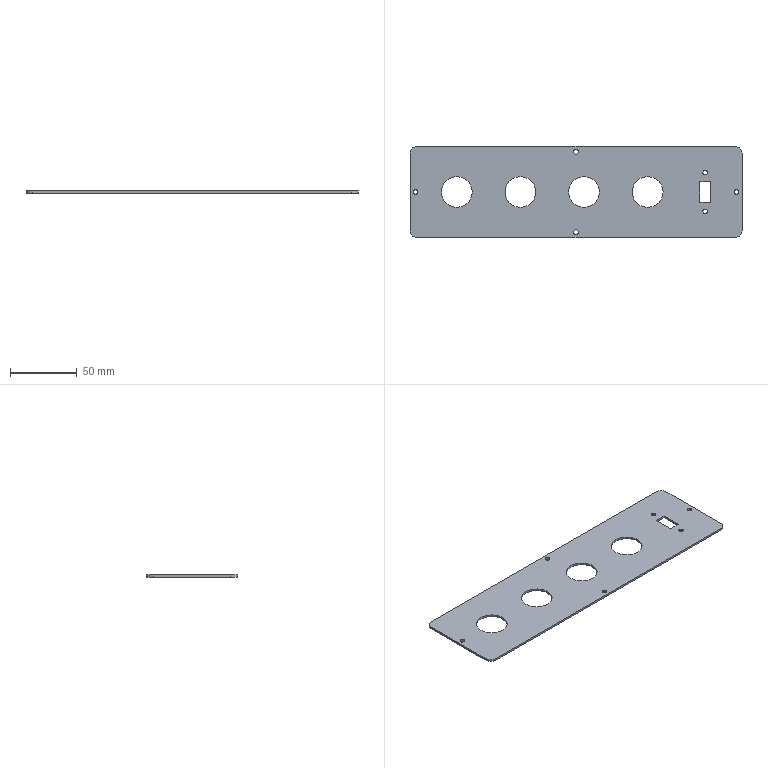Part | STEP file | FHD-021-005 power button plate | 1 solid | 24 faces | box 248 x 68 x 1.5 mm | volume 22504 mm3 | cylinder 14 | plane 10 | commonest cylinder face diameters 3.5 x6 10 x4 23 x4